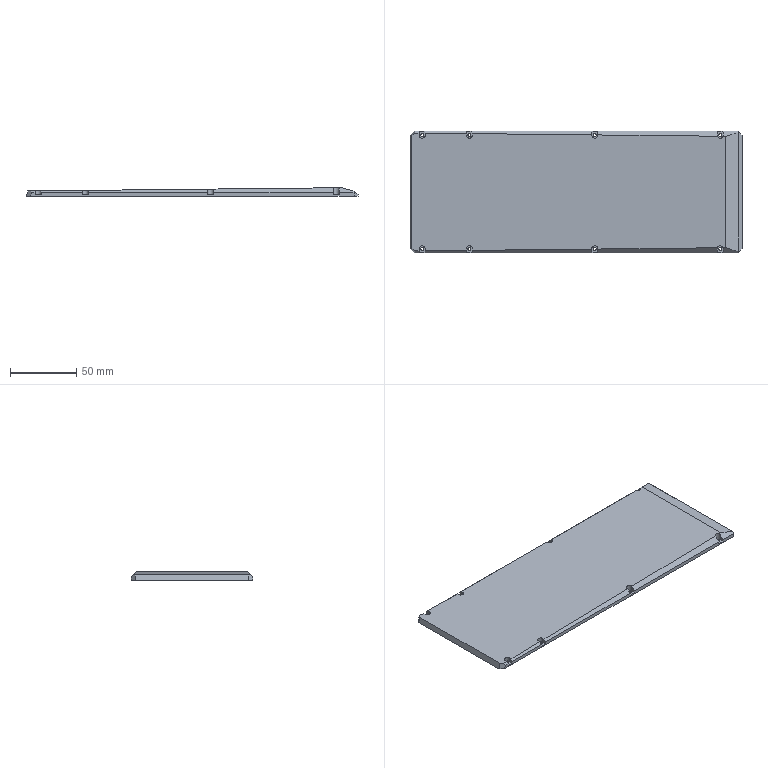NC program | NX | posted with a generic post | part box 251.5 x 92 x 6.5 mm
Whole program:
N10 G17 G21 G94 G90
(CURVE_DRIVE_COPY_COPY_COPY , TOOL : D4R0.5)
N12 T12 M6
N14 G54
N16 G17 G0 G90 X-42.956 Y127.252 S6000 M3
N18 G43 Z36.5 H12
N20 Z6.658
N22 G94 G1 Z5.365 F3000.
N24 X-43.06 Y127.142 Z4.758
N26 X-43.287 Y126.9 Z4.228
N28 X-43.615 Y126.55 Z3.826
N30 X-44.013 Y126.127 Z3.592
N32 X-44.44 Y125.672 Z3.548
N34 X-44.664 Y125.434 Z3.568
N36 X-44.846 Y125.241 Z3.564
N38 X-45.052 Y125.021 Z3.565
N40 X-45.286 Y124.772 Z3.578
N42 X-46.098 Y123.907 Z3.589
N44 X-46.199 Y123.8 Z3.562
N46 X-46.284 Y123.738 Z3.475
N48 X-46.14 Y123.891 Z3.511
N50 X-45.223 Y124.868 Z3.505
N52 X-45.078 Y125.021 Z3.496
N54 X-44.557 Y125.576 Z3.501
N56 X-44.443 Y125.698 Z3.487
N58 Y125.726 Z3.412
N60 X-44.57 Y125.59 Z3.433
N62 X-45.396 Y124.711 Z3.429
N64 X-46.182 Y123.875 Z3.433
N66 X-46.293 Y123.757 Z3.404
N68 X-46.355 Y123.691 Z3.407
N70 X-46.426 Y123.643 Z3.337
N72 X-46.308 Y123.768 Z3.336
N74 X-46.223 Y123.859 Z3.358
N76 X-44.57 Y125.618
N78 X-44.443 Y125.753 Z3.337
N80 Y125.78 Z3.262
N82 X-44.57 Y125.645 Z3.282
N84 X-46.263 Y123.843 Z3.283
N86 X-46.323 Y123.779 Z3.267
N88 X-46.446 Y123.649 Z3.272
N90 X-46.503 Y123.588 Z3.259
N92 X-46.572 Y123.542 Z3.192
N94 X-46.48 Y123.64 Z3.204
N96 X-46.339 Y123.79 Z3.199
N98 X-46.304 Y123.827 Z3.208
N100 X-44.57 Y125.672 Z3.207
N102 X-44.443 Y125.808 Z3.187
N104 Y125.835 Z3.112
N106 X-44.57 Y125.7 Z3.132
N108 X-46.521 Y123.624 Z3.133
N110 X-46.643 Y123.494 Z3.122
N112 X-46.72 Y123.439 Z3.045
N114 X-46.569 Y123.599 Z3.058
N116 X-44.57 Y125.727 Z3.057
N118 X-44.443 Y125.862 Z3.037
N120 Y125.89 Z2.961
N122 X-44.57 Y125.754 Z2.982
N124 X-46.618 Y123.575
N126 X-46.797 Y123.384 Z2.967
N128 X-46.871 Y123.333 Z2.894
N130 X-46.667 Y123.55 Z2.907
N132 X-44.57 Y125.782
N134 X-44.443 Y125.917 Z2.886
N136 Y125.944 Z2.811
N138 X-44.57 Y125.809 Z2.831
N140 X-46.716 Y123.526 Z2.832
N142 X-46.873 Y123.359 Z2.819
N144 X-46.942 Y123.285 Z2.824
N146 X-47.014 Y123.236 Z2.753
N148 X-46.898 Y123.359 Z2.746
N150 X-46.765 Y123.501 Z2.757
N152 X-44.57 Y125.837 Z2.756
N154 X-44.443 Y125.972 Z2.736
N156 Y125.999 Z2.661
N158 X-44.57 Y125.864 Z2.681
N160 X-46.813 Y123.477 Z2.682
N162 X-46.924 Y123.359 Z2.672
N164 X-47.071 Y123.203 Z2.68
N166 X-47.095 Y123.177 Z2.671
N168 X-47.174 Y123.12 Z2.59
N170 X-47.048 Y123.255 Z2.607
N172 X-46.95 Y123.359 Z2.599
N174 X-46.862 Y123.452 Z2.607
N176 X-44.57 Y125.891 Z2.606
N178 X-44.443 Y126.027 Z2.586
N180 Y126.054 Z2.51
N182 X-44.57 Y125.919 Z2.531
N184 X-46.911 Y123.428 Z2.532
N186 X-46.976 Y123.359 Z2.526
N188 X-47.087 Y123.24 Z2.532
N190 X-47.253 Y123.063 Z2.509
N192 X-47.334 Y123.005 Z2.428
N194 X-47.105 Y123.249 Z2.456
N196 X-44.57 Y125.946
N198 X-44.443 Y126.081 Z2.435
N200 Y126.109 Z2.36
N202 X-44.57 Y125.973 Z2.38
N204 X-47.122 Y123.258 Z2.381
N206 X-47.415 Y122.945 Z2.344
N208 X-47.44 Y122.927 Z2.32
N210 Y122.946 Z2.268
N212 X-47.14 Y123.266 Z2.306
N214 X-44.57 Y126.001 Z2.305
N216 X-44.443 Y126.136 Z2.285
N218 Y126.163 Z2.21
N220 X-44.57 Y126.028 Z2.23
N222 X-47.157 Y123.275 Z2.231
N224 X-47.44 Y122.973 Z2.195
N226 X-47.441 Y123. Z2.122
N228 X-47.174 Y123.284 Z2.156
N230 X-44.57 Y126.055 Z2.155
N232 X-44.443 Y126.191 Z2.135
N234 Y126.218 Z2.059
N236 X-44.57 Y126.083 Z2.08
N238 X-47.192 Y123.293 Z2.081
N240 X-47.441 Y123.027 Z2.049
N242 X-47.442 Y123.054 Z1.976
N244 X-47.209 Y123.301 Z2.005
N246 X-44.57 Y126.11
N248 X-44.443 Y126.245 Z1.984
N250 Y126.273 Z1.909
N252 X-44.57 Y126.137 Z1.929
N254 X-47.227 Y123.31 Z1.93
N256 X-47.442 Y123.081 Z1.903
N258 Y123.108 Z1.83
N260 X-47.244 Y123.319 Z1.855
N262 X-44.57 Y126.165 Z1.854
N264 X-44.443 Y126.3 Z1.834
N266 Y126.328 Z1.759
N268 X-44.57 Y126.192 Z1.779
N270 X-47.262 Y123.328 Z1.78
N272 X-47.442 Y123.135 Z1.756
N274 Y123.163 Z1.681
N276 X-47.279 Y123.337 Z1.705
N278 X-44.57 Y126.22 Z1.704
N280 X-44.443 Y126.355 Z1.683
N282 Y126.382 Z1.608
N284 X-44.57 Y126.247 Z1.629
N286 X-47.297 Y123.345 Z1.63
N288 X-47.442 Y123.19 Z1.606
N290 Y123.218 Z1.53
N292 X-47.314 Y123.354 Z1.554
N294 X-44.57 Y126.274 Z1.553
N296 X-44.443 Y126.41 Z1.533
N298 Y126.437 Z1.458
N300 X-44.57 Y126.302 Z1.478
N302 X-47.324 Y123.371 Z1.479
N304 X-47.442 Y123.245 Z1.455
N306 Y123.272 Z1.38
N308 X-47.326 Y123.396 Z1.404
N310 X-44.57 Y126.329 Z1.403
N312 X-44.443 Y126.464 Z1.383
N314 Y126.492 Z1.308
N316 X-44.57 Y126.356 Z1.328
N318 X-47.328 Y123.422 Z1.329
N320 X-47.442 Y123.3 Z1.305
N322 Y123.327 Z1.23
N324 X-47.329 Y123.447 Z1.254
N326 X-44.57 Y126.384 Z1.253
N328 X-44.443 Y126.519 Z1.232
N330 Y126.546 Z1.157
N332 X-44.57 Y126.411 Z1.178
N334 X-47.331 Y123.473 Z1.179
N336 X-47.442 Y123.355 Z1.155
N338 Y123.382 Z1.08
N340 X-47.333 Y123.498 Z1.103
N342 X-44.57 Y126.438 Z1.102
N344 X-44.443 Y126.574 Z1.082
N346 Y126.601 Z1.007
N348 X-44.57 Y126.466 Z1.027
N350 X-47.335 Y123.523 Z1.028
N352 X-47.442 Y123.409 Z1.005
N354 Y123.437 Z0.93
N356 X-47.337 Y123.549 Z0.953
N358 X-44.57 Y126.493 Z0.952
N360 X-44.443 Y126.628 Z0.932
N362 Y126.656 Z0.857
N364 X-44.57 Y126.521 Z0.877
N366 X-47.339 Y123.574 Z0.878
N368 X-47.442 Y123.464 Z0.855
N370 Y123.491 Z0.781
N372 X-47.341 Y123.599 Z0.803
N374 X-44.57 Y126.548 Z0.802
N376 X-44.443 Y126.683 Z0.781
N378 Y126.711 Z0.706
N380 X-44.57 Y126.575 Z0.727
N382 X-47.343 Y123.625
N384 X-47.442 Y123.518 Z0.706
N386 X-47.443 Y123.546 Z0.631
N388 X-47.344 Y123.65 Z0.652
N390 X-44.57 Y126.603 Z0.651
N392 X-44.443 Y126.738 Z0.631
N394 Y126.765 Z0.556
N396 X-44.57 Y126.63 Z0.576
N398 X-47.346 Y123.675 Z0.577
N400 X-47.443 Y123.573 Z0.556
N402 Y123.6 Z0.481
N404 X-47.348 Y123.701 Z0.502
N406 X-44.57 Y126.657 Z0.501
N408 X-44.443 Y126.793 Z0.481
N410 Y126.82 Z0.405
N412 X-44.571 Y126.684 Z0.426
N414 X-47.35 Y123.726 Z0.427
N416 X-47.443 Y123.628 Z0.407
N418 Y123.655 Z0.332
N420 X-47.352 Y123.752 Z0.352
N422 X-44.597 Y126.684 Z0.351
N424 X-44.443 Y126.847 Z0.33
N426 Y126.875 Z0.255
N428 X-44.622 Y126.684 Z0.275
N430 X-47.354 Y123.777 Z0.276
N432 X-47.443 Y123.682 Z0.257
N434 Y123.71 Z0.182
N436 X-47.356 Y123.802 Z0.201
N438 X-44.648 Y126.684 Z0.2
N440 X-44.443 Y126.902 Z0.18
N442 Y126.929 Z0.105
N444 X-44.674 Y126.684 Z0.126
N446 X-47.358 Y123.828
N448 X-47.443 Y123.737 Z0.108
N450 Y123.763 Z0.037
N452 X-47.359 Y123.852 Z0.055
N454 X-47.178 Y124.045
N456 X-47.135 Y124.091 Z0.048
N458 X-46.954 Y124.283 Z0.055
N460 X-44.698 Y126.684 Z0.054
N462 X-44.443 Y126.955 Z0.033
N464 Y126.981 Z-0.038
N466 X-44.722 Y126.684 Z-0.015
N468 X-46.903 Y124.362 Z-0.014
N470 X-47.048 Y124.208 Z-0.023
N472 X-47.182 Y124.066 Z-0.025
N474 X-47.249 Y123.994 Z-0.014
N476 X-47.361 Y123.875
N478 X-47.443 Y123.788 Z-0.033
N480 Y123.813 Z-0.103
N482 X-47.363 Y123.898 Z-0.083
N484 X-47.32 Y123.944
N486 X-47.229 Y124.04 Z-0.098
N488 X-47.048 Y124.234 Z-0.096
N490 X-46.852 Y124.442 Z-0.083
N492 X-44.745 Y126.684 Z-0.084
N494 X-44.442 Y127.007 Z-0.11
N496 Y127.032 Z-0.181
N498 X-44.769 Y126.684 Z-0.153
N500 X-45.113 Y126.317
N502 X-45.29 Y126.13 Z-0.161
N504 X-46.356 Y124.995 Z-0.16
N506 X-46.866 Y124.452 Z-0.157
N508 X-47.048 Y124.259 Z-0.169
N510 X-47.276 Y124.015 Z-0.171
N512 X-47.373 Y123.913 Z-0.155
N514 X-47.443 Y123.839 Z-0.173
N516 X-47.442 Y123.864 Z-0.244
N518 X-47.396 Y123.913 Z-0.232
N520 X-47.324 Y123.99 Z-0.243
N522 X-47.048 Y124.284 Z-0.241
N524 X-46.876 Y124.467 Z-0.234
N526 X-45.834 Y125.576 Z-0.241
N528 X-45.313 Y126.13 Z-0.235
N530 X-45.031 Y126.43 Z-0.222
N532 X-44.792 Y126.684
N534 X-44.442 Y127.058 Z-0.252
N536 X-44.441 Y127.083 Z-0.323
N538 X-44.816 Y126.684 Z-0.291
N540 X-44.949 Y126.542
N542 X-45.396 Y126.067 Z-0.311
N544 X-45.947 Y125.481 Z-0.318
N546 X-46.955 Y124.407 Z-0.307
N548 X-47.048 Y124.309 Z-0.313
N550 X-47.37 Y123.965 Z-0.316
N552 X-47.42 Y123.913 Z-0.308
N554 X-47.442 Y123.889 Z-0.314
N556 Y123.913 Z-0.38
N558 X-45.319 Y126.175 Z-0.382
N560 X-44.84 Y126.684 Z-0.361
N562 X-44.742 Y126.788 Z-0.369
N564 X-44.675 Y126.86 Z-0.382
N566 X-44.247 Y127.315 Z-0.364
N568 X-43.843 Y127.745 Z-0.154
N570 X-43.504 Y128.106 Z0.229
N572 X-43.262 Y128.363 Z0.745
N574 X-43.142 Y128.492 Z1.346
N576 Z5.683
N578 G0 Z36.5
N580 X47.734 Y122.163
N582 Z6.628
N584 G1 Z5.214
N586 X47.597 Y122.31 Z4.622
N588 X47.34 Y122.583 Z4.12
N590 X46.99 Y122.955 Z3.76
N592 X46.581 Y123.391 Z3.574
N594 X46.152 Y123.847 Z3.583
N596 X46.092 Y123.911 Z3.598
N598 X45.296 Y124.758 Z3.588
N600 X45.047 Y125.022 Z3.574
N602 X44.674 Y125.419 Z3.577
N604 X44.527 Y125.577 Z3.568
N606 X44.439 Y125.669 Z3.557
N608 X44.442 Y125.695 Z3.494
N610 X44.611 Y125.515 Z3.512
N612 X45.074 Y125.022 Z3.505
N614 X45.232 Y124.854 Z3.514
N616 X46.134 Y123.894 Z3.52
N618 X46.245 Y123.776 Z3.492
N620 X46.324 Y123.719 Z3.417
N622 X46.29 Y123.756 Z3.416
N624 X46.174 Y123.879 Z3.446
N626 X45.099 Y125.022 Z3.439
N628 X44.57 Y125.586 Z3.446
N630 X44.443 Y125.721 Z3.426
N632 Y125.748 Z3.351
N634 X44.57 Y125.613 Z3.371
N636 X46.215 Y123.863
N638 X46.305 Y123.767 Z3.348
N640 X46.397 Y123.669 Z3.351
N642 X46.477 Y123.611 Z3.274
N644 X46.439 Y123.651 Z3.283
N646 X46.32 Y123.778 Z3.279
N648 X46.255 Y123.847 Z3.296
N650 X44.57 Y125.64
N652 X44.443 Y125.776 Z3.275
N654 Y125.803 Z3.2
N656 X44.57 Y125.668 Z3.221
N658 X46.295 Y123.832 Z3.22
N660 X46.335 Y123.789 Z3.21
N662 X46.473 Y123.643 Z3.215
N664 X46.553 Y123.557 Z3.204
N666 X46.626 Y123.507 Z3.137
N668 X46.452 Y123.693 Z3.145
N670 X46.155 Y124.009
N672 X44.57 Y125.695
N674 X44.443 Y125.83 Z3.125
N676 Y125.858 Z3.05
N678 X44.57 Y125.722 Z3.07
N680 X46.56 Y123.605
N682 X46.707 Y123.448 Z3.058
N684 X46.784 Y123.394 Z2.981
N686 X46.609 Y123.581 Z2.995
N688 X44.57 Y125.75
N690 X44.443 Y125.885 Z2.975
N692 Y125.913 Z2.9
N694 X44.57 Y125.777 Z2.92
N696 X46.657 Y123.556
N698 X46.859 Y123.342 Z2.906
N700 X46.93 Y123.293 Z2.836
N702 X46.868 Y123.36 Z2.831
N704 X46.706 Y123.531 Z2.845
N706 X44.57 Y125.804
N708 X44.443 Y125.94 Z2.824
N710 Y125.967 Z2.749
N712 X44.57 Y125.832 Z2.77
N714 X46.755 Y123.507 Z2.769
N716 X46.893 Y123.36 Z2.758
N718 X47.001 Y123.245 Z2.766
N720 X47.081 Y123.187 Z2.684
N722 X47.048 Y123.223 Z2.694
N724 X46.919 Y123.36 Z2.685
N726 X46.804 Y123.482 Z2.694
N728 X44.57 Y125.859
N730 X44.443 Y125.995 Z2.674
N732 Y126.022 Z2.599
N734 X44.57 Y125.887 Z2.619
N736 X46.852 Y123.458
N738 X46.945 Y123.36 Z2.611
N740 X47.066 Y123.23 Z2.619
N742 X47.161 Y123.13 Z2.603
N744 X47.239 Y123.073 Z2.522
N746 X47.084 Y123.239 Z2.544
N748 X46.971 Y123.36 Z2.538
N750 X46.901 Y123.433 Z2.544
N752 X44.57 Y125.914
N754 X44.443 Y126.049 Z2.524
N756 Y126.077 Z2.449
N758 X44.57 Y125.941 Z2.469
N760 X46.996 Y123.36 Z2.465
N762 X47.101 Y123.248 Z2.469
N764 X47.318 Y123.017 Z2.441
N766 X47.4 Y122.958 Z2.358
N768 X47.119 Y123.257 Z2.394
N770 X44.57 Y125.969
N772 X44.443 Y126.104 Z2.373
N774 Y126.131 Z2.3
N776 X44.57 Y125.996 Z2.319
N778 X47.136 Y123.266 Z2.318
N780 X47.44 Y122.942 Z2.28
N782 X47.441 Y122.969 Z2.207
N784 X47.154 Y123.274 Z2.243
N786 X44.57 Y126.023
N788 X44.443 Y126.159 Z2.223
N790 Y126.186 Z2.148
N792 X44.57 Y126.051 Z2.168
N794 X47.171 Y123.283
N796 X47.441 Y122.996 Z2.134
N798 Y123.023 Z2.061
N800 X47.188 Y123.292 Z2.093
N802 X44.57 Y126.078
N804 X44.443 Y126.213 Z2.073
N806 Y126.241 Z1.997
N808 X44.57 Y126.105 Z2.018
N810 X47.206 Y123.301
N812 X47.442 Y123.05 Z1.988
N814 Y123.077 Z1.915
N816 X47.223 Y123.309 Z1.942
N818 X44.57 Y126.133 Z1.943
N820 X44.443 Y126.268 Z1.922
N822 Y126.296 Z1.847
N824 X44.57 Y126.16 Z1.867
N826 X47.241 Y123.318
N828 X47.442 Y123.104 Z1.842
N830 X47.443 Y123.131 Z1.768
N832 X47.258 Y123.327 Z1.792
N834 X44.57 Y126.188
N836 X44.443 Y126.323 Z1.772
N838 Y126.35 Z1.697
N840 X44.57 Y126.215 Z1.717
N842 X47.276 Y123.336
N844 X47.442 Y123.158 Z1.693
N846 Y123.186 Z1.618
N848 X47.293 Y123.345 Z1.642
N850 X44.57 Y126.242
N852 X44.443 Y126.378 Z1.622
N854 Y126.405 Z1.546
N856 X44.57 Y126.27 Z1.567
N858 X47.311 Y123.353
N860 X47.442 Y123.213 Z1.542
N862 Y123.24 Z1.467
N864 X47.325 Y123.365 Z1.491
N866 X44.57 Y126.297 Z1.492
N868 X44.443 Y126.432 Z1.471
N870 Y126.46 Z1.396
N872 X44.57 Y126.324 Z1.416
N874 X47.333 Y123.384
N876 X47.442 Y123.268 Z1.392
N878 Y123.295 Z1.317
N880 X47.342 Y123.402 Z1.341
N882 X44.57 Y126.352
N884 X44.443 Y126.487 Z1.321
N886 Y126.514 Z1.246
N888 X44.57 Y126.379 Z1.266
N890 X47.351 Y123.42
N892 X47.442 Y123.323 Z1.242
N894 Y123.35 Z1.167
N896 X47.359 Y123.439 Z1.19
N898 X44.57 Y126.406 Z1.191
N900 X44.443 Y126.542 Z1.171
N902 Y126.569 Z1.095
N904 X44.57 Y126.434 Z1.116
N906 X47.368 Y123.457 Z1.115
N908 X47.443 Y123.377 Z1.093
N910 Y123.404 Z1.02
N912 X47.376 Y123.475 Z1.04
N914 X44.57 Y126.461 Z1.041
N916 X44.443 Y126.597 Z1.02
N918 Y126.624 Z0.945
N920 X44.57 Y126.488 Z0.965
N922 X47.384 Y123.494
N924 X47.443 Y123.431 Z0.947
N926 X47.444 Y123.458 Z0.874
N928 X47.393 Y123.512 Z0.89
N930 X44.57 Y126.516
N932 X44.443 Y126.651 Z0.87
N934 Y126.679 Z0.795
N936 X44.57 Y126.543 Z0.815
N938 X47.401 Y123.531 Z0.814
N940 X47.444 Y123.485 Z0.802
N942 X47.445 Y123.512 Z0.729
N944 X47.41 Y123.549 Z0.739
N946 X44.57 Y126.571 Z0.74
N948 X44.443 Y126.706 Z0.72
N950 Y126.733 Z0.644
N952 X44.57 Y126.598 Z0.665
N954 X47.418 Y123.567 Z0.664
N956 X47.445 Y123.539 Z0.656
N958 Y123.566 Z0.583
N960 X47.427 Y123.586 Z0.589
N962 X44.57 Y126.625 Z0.59
N964 X44.443 Y126.761 Z0.569
N966 Y126.788 Z0.494
N968 X44.57 Y126.653 Z0.514
N970 X47.435 Y123.604 Z0.513
N972 X47.446 Y123.592 Z0.51
N974 Y123.619 Z0.437
N976 X44.569 Y126.682 Z0.439
N978 X44.443 Y126.815 Z0.419
N980 Y126.843 Z0.344
N982 X44.591 Y126.685 Z0.364
N984 X47.446 Y123.647 Z0.363
N986 Y123.674 Z0.288
N988 X44.617 Y126.685 Z0.289
N990 X44.443 Y126.87 Z0.268
N992 Y126.898 Z0.193
N994 X44.643 Y126.685 Z0.214
N996 X47.446 Y123.701 Z0.213
N998 Y123.729 Z0.137
N1000 X44.668 Y126.685 Z0.138
N1002 X44.443 Y126.925 Z0.118
N1004 Y126.952 Z0.043
N1006 X44.694 Y126.685 Z0.064
N1008 X47.446 Y123.756 Z0.061
N1010 Y123.783 Z-0.014
N1012 X47.399 Y123.833 Z-0.01
N1014 X44.719 Y126.685 Z-0.009
N1016 X44.442 Y126.979 Z-0.032
N1018 Y127.006 Z-0.108
N1020 X44.744 Y126.685 Z-0.082
N1022 X47.377 Y123.882 Z-0.083
N1024 X47.445 Y123.81 Z-0.089
N1026 X47.444 Y123.837 Z-0.164
N1028 X47.372 Y123.914 Z-0.156
N1030 X45.289 Y126.131 Z-0.162
N1032 X45.116 Y126.314 Z-0.153
N1034 X44.768 Y126.685
N1036 X44.442 Y127.032 Z-0.18
N1038 X44.441 Y127.057 Z-0.249
N1040 X44.791 Y126.685 Z-0.22
N1042 X45.036 Y126.424
N1044 X45.312 Y126.131 Z-0.235
N1046 X46.473 Y124.895 Z-0.229
N1048 X46.497 Y124.869 Z-0.236
N1050 X47.395 Y123.914 Z-0.232
N1052 X47.443 Y123.863 Z-0.238
N1054 X47.441 Y123.889 Z-0.311
N1056 X46.951 Y124.41 Z-0.306
N1058 X46.897 Y124.468 Z-0.312
N1060 X46.497 Y124.894
N1062 X46.458 Y124.935 Z-0.302
N1064 X45.334 Y126.131 Z-0.308
N1066 X44.957 Y126.533 Z-0.287
N1068 X44.814 Y126.685 Z-0.286
N1070 X44.441 Y127.082 Z-0.318
N1072 X44.439 Y127.103 Z-0.382
N1074 X44.589 Y126.949
N1076 X44.679 Y126.852 Z-0.367
N1078 X44.877 Y126.642 Z-0.353
N1080 X45.391 Y126.095 Z-0.382
N1082 X45.54 Y125.937
N1084 X46.443 Y124.975 Z-0.375
N1086 X46.472 Y124.945 Z-0.382
N1088 X46.98 Y124.404
N1090 X47.193 Y124.178
N1092 X47.617 Y123.726 Z-0.29
N1094 X48. Y123.318 Z-0.011
N1096 X48.306 Y122.993 Z0.427
N1098 X48.504 Y122.782 Z0.982
N1100 X48.576 Y122.706 Z1.599
N1102 Z6.022
N1104 G0 Z36.5
N1106 M5
N1108 M2